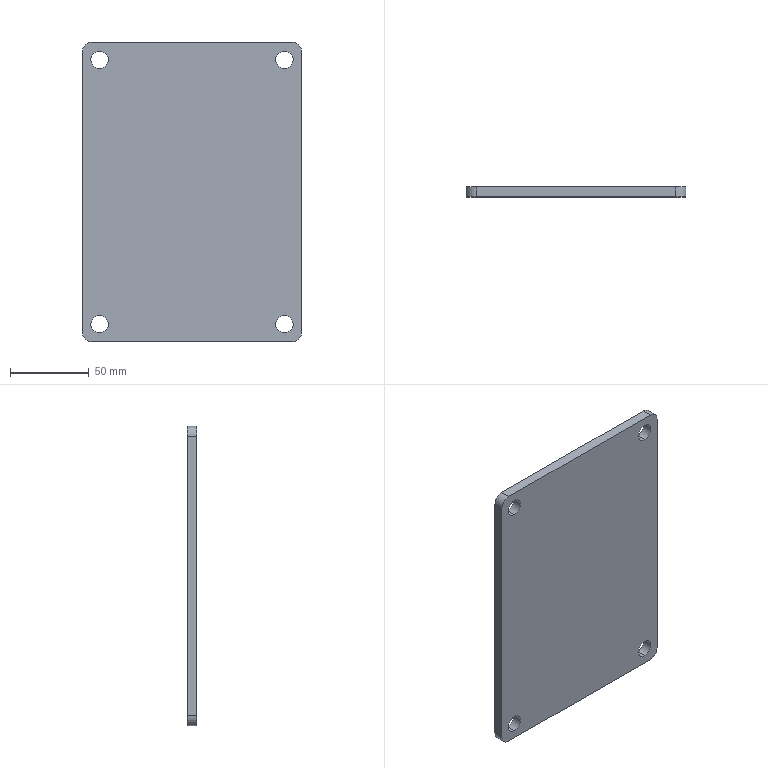Part | SolidWorks | features Extrusion 1, Fillet 1, HoleWzd 1, LPattern 1 | 1 solid | 18 faces | box 139.7 x 6.35 x 190.5 mm | volume 166308 mm3 | cylinder 12 | plane 6 | commonest cylinder face diameters 11.112 x8 12.7 x4
STEP:
#1=CARTESIAN_POINT('',(58.737,0.,78.581));
#2=VERTEX_POINT('',#1);
#3=CARTESIAN_POINT('',(58.737,0.,89.693));
#4=VERTEX_POINT('',#3);
#5=CARTESIAN_POINT('',(58.737,0.,84.137));
#6=DIRECTION('',(0.,1.,0.));
#7=DIRECTION('',(0.,0.,1.));
#8=AXIS2_PLACEMENT_3D('',#5,#6,#7);
#9=CIRCLE('',#8,5.556);
#10=EDGE_CURVE('',#2,#4,#9,.T.);
#11=ORIENTED_EDGE('',*,*,#10,.F.);
#12=CARTESIAN_POINT('',(58.737,6.35,78.581));
#13=VERTEX_POINT('',#12);
#14=CARTESIAN_POINT('',(58.737,6.35,78.581));
#15=DIRECTION('',(0.,1.,0.));
#16=VECTOR('',#15,1000.);
#17=LINE('',#14,#16);
#18=EDGE_CURVE('',#2,#13,#17,.T.);
#19=ORIENTED_EDGE('',*,*,#18,.T.);
#20=CARTESIAN_POINT('',(58.737,6.35,89.693));
#21=VERTEX_POINT('',#20);
#22=CARTESIAN_POINT('',(58.737,6.35,84.137));
#23=DIRECTION('',(0.,1.,0.));
#24=DIRECTION('',(0.,0.,1.));
#25=AXIS2_PLACEMENT_3D('',#22,#23,#24);
#26=CIRCLE('',#25,5.556);
#27=EDGE_CURVE('',#13,#21,#26,.T.);
#28=ORIENTED_EDGE('',*,*,#27,.T.);
#29=CARTESIAN_POINT('',(58.737,6.35,89.693));
#30=DIRECTION('',(0.,1.,0.));
#31=VECTOR('',#30,1000.);
#32=LINE('',#29,#31);
#33=EDGE_CURVE('',#4,#21,#32,.T.);
#34=ORIENTED_EDGE('',*,*,#33,.F.);
#35=EDGE_LOOP('',(#11,#19,#28,#34));
#36=FACE_OUTER_BOUND('',#35,.T.);
#37=CARTESIAN_POINT('',(58.737,6.35,84.137));
#38=DIRECTION('',(0.,1.,0.));
#39=DIRECTION('',(0.,0.,1.));
#40=AXIS2_PLACEMENT_3D('',#37,#38,#39);
#41=CYLINDRICAL_SURFACE('',#40,5.556);
#42=ADVANCED_FACE('',(#36),#41,.F.);
#43=CARTESIAN_POINT('',(-58.738,0.,78.581));
#44=VERTEX_POINT('',#43);
#45=CARTESIAN_POINT('',(-58.738,0.,89.693));
#46=VERTEX_POINT('',#45);
#47=CARTESIAN_POINT('',(-58.738,0.,84.137));
#48=DIRECTION('',(0.,1.,0.));
#49=DIRECTION('',(0.,0.,1.));
#50=AXIS2_PLACEMENT_3D('',#47,#48,#49);
#51=CIRCLE('',#50,5.556);
#52=EDGE_CURVE('',#44,#46,#51,.T.);
#53=ORIENTED_EDGE('',*,*,#52,.F.);
#54=CARTESIAN_POINT('',(-58.738,6.35,78.581));
#55=VERTEX_POINT('',#54);
#56=CARTESIAN_POINT('',(-58.738,6.35,78.581));
#57=DIRECTION('',(0.,1.,0.));
#58=VECTOR('',#57,1000.);
#59=LINE('',#56,#58);
#60=EDGE_CURVE('',#44,#55,#59,.T.);
#61=ORIENTED_EDGE('',*,*,#60,.T.);
#62=CARTESIAN_POINT('',(-58.738,6.35,89.693));
#63=VERTEX_POINT('',#62);
#64=CARTESIAN_POINT('',(-58.738,6.35,84.137));
#65=DIRECTION('',(0.,1.,0.));
#66=DIRECTION('',(0.,0.,1.));
#67=AXIS2_PLACEMENT_3D('',#64,#65,#66);
#68=CIRCLE('',#67,5.556);
#69=EDGE_CURVE('',#55,#63,#68,.T.);
#70=ORIENTED_EDGE('',*,*,#69,.T.);
#71=CARTESIAN_POINT('',(-58.738,6.35,89.693));
#72=DIRECTION('',(0.,1.,0.));
#73=VECTOR('',#72,1000.);
#74=LINE('',#71,#73);
#75=EDGE_CURVE('',#46,#63,#74,.T.);
#76=ORIENTED_EDGE('',*,*,#75,.F.);
#77=EDGE_LOOP('',(#53,#61,#70,#76));
#78=FACE_OUTER_BOUND('',#77,.T.);
#79=CARTESIAN_POINT('',(-58.738,6.35,84.137));
#80=DIRECTION('',(0.,1.,0.));
#81=DIRECTION('',(0.,0.,1.));
#82=AXIS2_PLACEMENT_3D('',#79,#80,#81);
#83=CYLINDRICAL_SURFACE('',#82,5.556);
#84=ADVANCED_FACE('',(#78),#83,.F.);
#85=CARTESIAN_POINT('',(58.737,0.,-89.694));
#86=VERTEX_POINT('',#85);
#87=CARTESIAN_POINT('',(58.737,0.,-78.582));
#88=VERTEX_POINT('',#87);
#89=CARTESIAN_POINT('',(58.737,0.,-84.138));
#90=DIRECTION('',(0.,1.,0.));
#91=DIRECTION('',(0.,0.,1.));
#92=AXIS2_PLACEMENT_3D('',#89,#90,#91);
#93=CIRCLE('',#92,5.556);
#94=EDGE_CURVE('',#86,#88,#93,.T.);
#95=ORIENTED_EDGE('',*,*,#94,.F.);
#96=CARTESIAN_POINT('',(58.737,6.35,-89.694));
#97=VERTEX_POINT('',#96);
#98=CARTESIAN_POINT('',(58.737,6.35,-89.694));
#99=DIRECTION('',(0.,1.,0.));
#100=VECTOR('',#99,1000.);
#101=LINE('',#98,#100);
#102=EDGE_CURVE('',#86,#97,#101,.T.);
#103=ORIENTED_EDGE('',*,*,#102,.T.);
#104=CARTESIAN_POINT('',(58.737,6.35,-78.582));
#105=VERTEX_POINT('',#104);
#106=CARTESIAN_POINT('',(58.737,6.35,-84.138));
#107=DIRECTION('',(0.,1.,0.));
#108=DIRECTION('',(0.,0.,1.));
#109=AXIS2_PLACEMENT_3D('',#106,#107,#108);
#110=CIRCLE('',#109,5.556);
#111=EDGE_CURVE('',#97,#105,#110,.T.);
#112=ORIENTED_EDGE('',*,*,#111,.T.);
#113=CARTESIAN_POINT('',(58.737,6.35,-78.582));
#114=DIRECTION('',(0.,1.,0.));
#115=VECTOR('',#114,1000.);
#116=LINE('',#113,#115);
#117=EDGE_CURVE('',#88,#105,#116,.T.);
#118=ORIENTED_EDGE('',*,*,#117,.F.);
#119=EDGE_LOOP('',(#95,#103,#112,#118));
#120=FACE_OUTER_BOUND('',#119,.T.);
#121=CARTESIAN_POINT('',(58.737,6.35,-84.138));
#122=DIRECTION('',(0.,1.,0.));
#123=DIRECTION('',(0.,0.,1.));
#124=AXIS2_PLACEMENT_3D('',#121,#122,#123);
#125=CYLINDRICAL_SURFACE('',#124,5.556);
#126=ADVANCED_FACE('',(#120),#125,.F.);
#127=CARTESIAN_POINT('',(-58.738,0.,-89.694));
#128=VERTEX_POINT('',#127);
#129=CARTESIAN_POINT('',(-58.738,0.,-78.582));
#130=VERTEX_POINT('',#129);
#131=CARTESIAN_POINT('',(-58.738,0.,-84.138));
#132=DIRECTION('',(0.,1.,0.));
#133=DIRECTION('',(0.,0.,1.));
#134=AXIS2_PLACEMENT_3D('',#131,#132,#133);
#135=CIRCLE('',#134,5.556);
#136=EDGE_CURVE('',#128,#130,#135,.T.);
#137=ORIENTED_EDGE('',*,*,#136,.F.);
#138=CARTESIAN_POINT('',(-58.738,6.35,-89.694));
#139=VERTEX_POINT('',#138);
#140=CARTESIAN_POINT('',(-58.738,6.35,-89.694));
#141=DIRECTION('',(0.,1.,0.));
#142=VECTOR('',#141,1000.);
#143=LINE('',#140,#142);
#144=EDGE_CURVE('',#128,#139,#143,.T.);
#145=ORIENTED_EDGE('',*,*,#144,.T.);
#146=CARTESIAN_POINT('',(-58.738,6.35,-78.582));
#147=VERTEX_POINT('',#146);
#148=CARTESIAN_POINT('',(-58.738,6.35,-84.138));
#149=DIRECTION('',(0.,1.,0.));
#150=DIRECTION('',(0.,0.,1.));
#151=AXIS2_PLACEMENT_3D('',#148,#149,#150);
#152=CIRCLE('',#151,5.556);
#153=EDGE_CURVE('',#139,#147,#152,.T.);
#154=ORIENTED_EDGE('',*,*,#153,.T.);
#155=CARTESIAN_POINT('',(-58.738,6.35,-78.582));
#156=DIRECTION('',(0.,1.,0.));
#157=VECTOR('',#156,1000.);
#158=LINE('',#155,#157);
#159=EDGE_CURVE('',#130,#147,#158,.T.);
#160=ORIENTED_EDGE('',*,*,#159,.F.);
#161=EDGE_LOOP('',(#137,#145,#154,#160));
#162=FACE_OUTER_BOUND('',#161,.T.);
#163=CARTESIAN_POINT('',(-58.738,6.35,-84.138));
#164=DIRECTION('',(0.,1.,0.));
#165=DIRECTION('',(0.,0.,1.));
#166=AXIS2_PLACEMENT_3D('',#163,#164,#165);
#167=CYLINDRICAL_SURFACE('',#166,5.556);
#168=ADVANCED_FACE('',(#162),#167,.F.);
#169=CARTESIAN_POINT('',(-69.85,6.35,-88.9));
#170=VERTEX_POINT('',#169);
#171=CARTESIAN_POINT('',(-69.85,6.35,88.9));
#172=VERTEX_POINT('',#171);
#173=CARTESIAN_POINT('',(-69.85,6.35,-95.25));
#174=DIRECTION('',(0.,0.,1.));
#175=VECTOR('',#174,1000.);
#176=LINE('',#173,#175);
#177=EDGE_CURVE('',#170,#172,#176,.T.);
#178=ORIENTED_EDGE('',*,*,#177,.F.);
#179=CARTESIAN_POINT('',(-69.85,0.,-88.9));
#180=VERTEX_POINT('',#179);
#181=CARTESIAN_POINT('',(-69.85,6.35,-88.9));
#182=DIRECTION('',(0.,-1.,0.));
#183=VECTOR('',#182,1000.);
#184=LINE('',#181,#183);
#185=EDGE_CURVE('',#170,#180,#184,.T.);
#186=ORIENTED_EDGE('',*,*,#185,.T.);
#187=CARTESIAN_POINT('',(-69.85,0.,88.9));
#188=VERTEX_POINT('',#187);
#189=CARTESIAN_POINT('',(-69.85,0.,-95.25));
#190=DIRECTION('',(0.,0.,1.));
#191=VECTOR('',#190,1000.);
#192=LINE('',#189,#191);
#193=EDGE_CURVE('',#180,#188,#192,.T.);
#194=ORIENTED_EDGE('',*,*,#193,.T.);
#195=CARTESIAN_POINT('',(-69.85,6.35,88.9));
#196=DIRECTION('',(0.,1.,0.));
#197=VECTOR('',#196,1000.);
#198=LINE('',#195,#197);
#199=EDGE_CURVE('',#188,#172,#198,.T.);
#200=ORIENTED_EDGE('',*,*,#199,.T.);
#201=EDGE_LOOP('',(#178,#186,#194,#200));
#202=FACE_OUTER_BOUND('',#201,.T.);
#203=CARTESIAN_POINT('',(-69.85,6.35,-95.25));
#204=DIRECTION('',(1.,0.,0.));
#205=DIRECTION('',(0.,0.,-1.));
#206=AXIS2_PLACEMENT_3D('',#203,#204,#205);
#207=PLANE('',#206);
#208=ADVANCED_FACE('',(#202),#207,.F.);
#209=CARTESIAN_POINT('',(-63.5,0.,95.25));
#210=VERTEX_POINT('',#209);
#211=CARTESIAN_POINT('',(63.5,0.,95.25));
#212=VERTEX_POINT('',#211);
#213=CARTESIAN_POINT('',(-69.85,0.,95.25));
#214=DIRECTION('',(1.,0.,0.));
#215=VECTOR('',#214,1000.);
#216=LINE('',#213,#215);
#217=EDGE_CURVE('',#210,#212,#216,.T.);
#218=ORIENTED_EDGE('',*,*,#217,.T.);
#219=CARTESIAN_POINT('',(63.5,6.35,95.25));
#220=VERTEX_POINT('',#219);
#221=CARTESIAN_POINT('',(63.5,6.35,95.25));
#222=DIRECTION('',(0.,1.,0.));
#223=VECTOR('',#222,1000.);
#224=LINE('',#221,#223);
#225=EDGE_CURVE('',#212,#220,#224,.T.);
#226=ORIENTED_EDGE('',*,*,#225,.T.);
#227=CARTESIAN_POINT('',(-63.5,6.35,95.25));
#228=VERTEX_POINT('',#227);
#229=CARTESIAN_POINT('',(-69.85,6.35,95.25));
#230=DIRECTION('',(1.,0.,0.));
#231=VECTOR('',#230,1000.);
#232=LINE('',#229,#231);
#233=EDGE_CURVE('',#228,#220,#232,.T.);
#234=ORIENTED_EDGE('',*,*,#233,.F.);
#235=CARTESIAN_POINT('',(-63.5,6.35,95.25));
#236=DIRECTION('',(0.,-1.,0.));
#237=VECTOR('',#236,1000.);
#238=LINE('',#235,#237);
#239=EDGE_CURVE('',#228,#210,#238,.T.);
#240=ORIENTED_EDGE('',*,*,#239,.T.);
#241=EDGE_LOOP('',(#218,#226,#234,#240));
#242=FACE_OUTER_BOUND('',#241,.T.);
#243=CARTESIAN_POINT('',(-69.85,6.35,95.25));
#244=DIRECTION('',(0.,0.,-1.));
#245=DIRECTION('',(-1.,0.,0.));
#246=AXIS2_PLACEMENT_3D('',#243,#244,#245);
#247=PLANE('',#246);
#248=ADVANCED_FACE('',(#242),#247,.F.);
#249=CARTESIAN_POINT('',(69.85,0.,88.9));
#250=VERTEX_POINT('',#249);
#251=CARTESIAN_POINT('',(69.85,0.,-88.9));
#252=VERTEX_POINT('',#251);
#253=CARTESIAN_POINT('',(69.85,0.,-95.25));
#254=DIRECTION('',(0.,0.,-1.));
#255=VECTOR('',#254,1000.);
#256=LINE('',#253,#255);
#257=EDGE_CURVE('',#250,#252,#256,.T.);
#258=ORIENTED_EDGE('',*,*,#257,.T.);
#259=CARTESIAN_POINT('',(69.85,6.35,-88.9));
#260=VERTEX_POINT('',#259);
#261=CARTESIAN_POINT('',(69.85,6.35,-88.9));
#262=DIRECTION('',(0.,1.,0.));
#263=VECTOR('',#262,1000.);
#264=LINE('',#261,#263);
#265=EDGE_CURVE('',#252,#260,#264,.T.);
#266=ORIENTED_EDGE('',*,*,#265,.T.);
#267=CARTESIAN_POINT('',(69.85,6.35,88.9));
#268=VERTEX_POINT('',#267);
#269=CARTESIAN_POINT('',(69.85,6.35,-95.25));
#270=DIRECTION('',(0.,0.,-1.));
#271=VECTOR('',#270,1000.);
#272=LINE('',#269,#271);
#273=EDGE_CURVE('',#268,#260,#272,.T.);
#274=ORIENTED_EDGE('',*,*,#273,.F.);
#275=CARTESIAN_POINT('',(69.85,6.35,88.9));
#276=DIRECTION('',(0.,-1.,0.));
#277=VECTOR('',#276,1000.);
#278=LINE('',#275,#277);
#279=EDGE_CURVE('',#268,#250,#278,.T.);
#280=ORIENTED_EDGE('',*,*,#279,.T.);
#281=EDGE_LOOP('',(#258,#266,#274,#280));
#282=FACE_OUTER_BOUND('',#281,.T.);
#283=CARTESIAN_POINT('',(69.85,6.35,-95.25));
#284=DIRECTION('',(-1.,0.,0.));
#285=DIRECTION('',(0.,0.,1.));
#286=AXIS2_PLACEMENT_3D('',#283,#284,#285);
#287=PLANE('',#286);
#288=ADVANCED_FACE('',(#282),#287,.F.);
#289=CARTESIAN_POINT('',(63.5,0.,-95.25));
#290=VERTEX_POINT('',#289);
#291=CARTESIAN_POINT('',(-63.5,0.,-95.25));
#292=VERTEX_POINT('',#291);
#293=CARTESIAN_POINT('',(-69.85,0.,-95.25));
#294=DIRECTION('',(-1.,0.,0.));
#295=VECTOR('',#294,1000.);
#296=LINE('',#293,#295);
#297=EDGE_CURVE('',#290,#292,#296,.T.);
#298=ORIENTED_EDGE('',*,*,#297,.T.);
#299=CARTESIAN_POINT('',(-63.5,6.35,-95.25));
#300=VERTEX_POINT('',#299);
#301=CARTESIAN_POINT('',(-63.5,6.35,-95.25));
#302=DIRECTION('',(0.,1.,0.));
#303=VECTOR('',#302,1000.);
#304=LINE('',#301,#303);
#305=EDGE_CURVE('',#292,#300,#304,.T.);
#306=ORIENTED_EDGE('',*,*,#305,.T.);
#307=CARTESIAN_POINT('',(63.5,6.35,-95.25));
#308=VERTEX_POINT('',#307);
#309=CARTESIAN_POINT('',(-69.85,6.35,-95.25));
#310=DIRECTION('',(-1.,0.,0.));
#311=VECTOR('',#310,1000.);
#312=LINE('',#309,#311);
#313=EDGE_CURVE('',#308,#300,#312,.T.);
#314=ORIENTED_EDGE('',*,*,#313,.F.);
#315=CARTESIAN_POINT('',(63.5,6.35,-95.25));
#316=DIRECTION('',(0.,-1.,0.));
#317=VECTOR('',#316,1000.);
#318=LINE('',#315,#317);
#319=EDGE_CURVE('',#308,#290,#318,.T.);
#320=ORIENTED_EDGE('',*,*,#319,.T.);
#321=EDGE_LOOP('',(#298,#306,#314,#320));
#322=FACE_OUTER_BOUND('',#321,.T.);
#323=CARTESIAN_POINT('',(-69.85,6.35,-95.25));
#324=DIRECTION('',(0.,0.,1.));
#325=DIRECTION('',(1.,0.,0.));
#326=AXIS2_PLACEMENT_3D('',#323,#324,#325);
#327=PLANE('',#326);
#328=ADVANCED_FACE('',(#322),#327,.F.);
#329=CARTESIAN_POINT('',(58.737,6.35,84.137));
#330=DIRECTION('',(0.,1.,0.));
#331=DIRECTION('',(0.,0.,1.));
#332=AXIS2_PLACEMENT_3D('',#329,#330,#331);
#333=CIRCLE('',#332,5.556);
#334=EDGE_CURVE('',#21,#13,#333,.T.);
#335=ORIENTED_EDGE('',*,*,#334,.F.);
#336=ORIENTED_EDGE('',*,*,#27,.F.);
#337=EDGE_LOOP('',(#335,#336));
#338=FACE_BOUND('',#337,.T.);
#339=CARTESIAN_POINT('',(-58.738,6.35,84.137));
#340=DIRECTION('',(0.,1.,0.));
#341=DIRECTION('',(0.,0.,1.));
#342=AXIS2_PLACEMENT_3D('',#339,#340,#341);
#343=CIRCLE('',#342,5.556);
#344=EDGE_CURVE('',#63,#55,#343,.T.);
#345=ORIENTED_EDGE('',*,*,#344,.F.);
#346=ORIENTED_EDGE('',*,*,#69,.F.);
#347=EDGE_LOOP('',(#345,#346));
#348=FACE_BOUND('',#347,.T.);
#349=CARTESIAN_POINT('',(58.737,6.35,-84.138));
#350=DIRECTION('',(0.,1.,0.));
#351=DIRECTION('',(0.,0.,1.));
#352=AXIS2_PLACEMENT_3D('',#349,#350,#351);
#353=CIRCLE('',#352,5.556);
#354=EDGE_CURVE('',#105,#97,#353,.T.);
#355=ORIENTED_EDGE('',*,*,#354,.F.);
#356=ORIENTED_EDGE('',*,*,#111,.F.);
#357=EDGE_LOOP('',(#355,#356));
#358=FACE_BOUND('',#357,.T.);
#359=CARTESIAN_POINT('',(-58.738,6.35,-84.138));
#360=DIRECTION('',(0.,1.,0.));
#361=DIRECTION('',(0.,0.,1.));
#362=AXIS2_PLACEMENT_3D('',#359,#360,#361);
#363=CIRCLE('',#362,5.556);
#364=EDGE_CURVE('',#147,#139,#363,.T.);
#365=ORIENTED_EDGE('',*,*,#364,.F.);
#366=ORIENTED_EDGE('',*,*,#153,.F.);
#367=EDGE_LOOP('',(#365,#366));
#368=FACE_BOUND('',#367,.T.);
#369=ORIENTED_EDGE('',*,*,#313,.T.);
#370=CARTESIAN_POINT('',(-63.5,6.35,-88.9));
#371=DIRECTION('',(0.,1.,0.));
#372=DIRECTION('',(0.,0.,1.));
#373=AXIS2_PLACEMENT_3D('',#370,#371,#372);
#374=CIRCLE('',#373,6.35);
#375=EDGE_CURVE('',#300,#170,#374,.T.);
#376=ORIENTED_EDGE('',*,*,#375,.T.);
#377=ORIENTED_EDGE('',*,*,#177,.T.);
#378=CARTESIAN_POINT('',(-63.5,6.35,88.9));
#379=DIRECTION('',(0.,1.,0.));
#380=DIRECTION('',(0.,0.,1.));
#381=AXIS2_PLACEMENT_3D('',#378,#379,#380);
#382=CIRCLE('',#381,6.35);
#383=EDGE_CURVE('',#172,#228,#382,.T.);
#384=ORIENTED_EDGE('',*,*,#383,.T.);
#385=ORIENTED_EDGE('',*,*,#233,.T.);
#386=CARTESIAN_POINT('',(63.5,6.35,88.9));
#387=DIRECTION('',(0.,1.,0.));
#388=DIRECTION('',(0.,0.,1.));
#389=AXIS2_PLACEMENT_3D('',#386,#387,#388);
#390=CIRCLE('',#389,6.35);
#391=EDGE_CURVE('',#220,#268,#390,.T.);
#392=ORIENTED_EDGE('',*,*,#391,.T.);
#393=ORIENTED_EDGE('',*,*,#273,.T.);
#394=CARTESIAN_POINT('',(63.5,6.35,-88.9));
#395=DIRECTION('',(0.,1.,0.));
#396=DIRECTION('',(0.,0.,1.));
#397=AXIS2_PLACEMENT_3D('',#394,#395,#396);
#398=CIRCLE('',#397,6.35);
#399=EDGE_CURVE('',#260,#308,#398,.T.);
#400=ORIENTED_EDGE('',*,*,#399,.T.);
#401=EDGE_LOOP('',(#369,#376,#377,#384,#385,#392,#393,#400));
#402=FACE_OUTER_BOUND('',#401,.T.);
#403=CARTESIAN_POINT('',(0.,6.35,0.));
#404=DIRECTION('',(0.,1.,0.));
#405=DIRECTION('',(0.,0.,1.));
#406=AXIS2_PLACEMENT_3D('',#403,#404,#405);
#407=PLANE('',#406);
#408=ADVANCED_FACE('',(#338,#348,#358,#368,#402),#407,.T.);
#409=CARTESIAN_POINT('',(58.737,0.,84.137));
#410=DIRECTION('',(0.,1.,0.));
#411=DIRECTION('',(0.,0.,1.));
#412=AXIS2_PLACEMENT_3D('',#409,#410,#411);
#413=CIRCLE('',#412,5.556);
#414=EDGE_CURVE('',#4,#2,#413,.T.);
#415=ORIENTED_EDGE('',*,*,#414,.T.);
#416=ORIENTED_EDGE('',*,*,#10,.T.);
#417=EDGE_LOOP('',(#415,#416));
#418=FACE_BOUND('',#417,.T.);
#419=CARTESIAN_POINT('',(-58.738,0.,84.137));
#420=DIRECTION('',(0.,1.,0.));
#421=DIRECTION('',(0.,0.,1.));
#422=AXIS2_PLACEMENT_3D('',#419,#420,#421);
#423=CIRCLE('',#422,5.556);
#424=EDGE_CURVE('',#46,#44,#423,.T.);
#425=ORIENTED_EDGE('',*,*,#424,.T.);
#426=ORIENTED_EDGE('',*,*,#52,.T.);
#427=EDGE_LOOP('',(#425,#426));
#428=FACE_BOUND('',#427,.T.);
#429=CARTESIAN_POINT('',(58.737,0.,-84.138));
#430=DIRECTION('',(0.,1.,0.));
#431=DIRECTION('',(0.,0.,1.));
#432=AXIS2_PLACEMENT_3D('',#429,#430,#431);
#433=CIRCLE('',#432,5.556);
#434=EDGE_CURVE('',#88,#86,#433,.T.);
#435=ORIENTED_EDGE('',*,*,#434,.T.);
#436=ORIENTED_EDGE('',*,*,#94,.T.);
#437=EDGE_LOOP('',(#435,#436));
#438=FACE_BOUND('',#437,.T.);
#439=CARTESIAN_POINT('',(-58.738,0.,-84.138));
#440=DIRECTION('',(0.,1.,0.));
#441=DIRECTION('',(0.,0.,1.));
#442=AXIS2_PLACEMENT_3D('',#439,#440,#441);
#443=CIRCLE('',#442,5.556);
#444=EDGE_CURVE('',#130,#128,#443,.T.);
#445=ORIENTED_EDGE('',*,*,#444,.T.);
#446=ORIENTED_EDGE('',*,*,#136,.T.);
#447=EDGE_LOOP('',(#445,#446));
#448=FACE_BOUND('',#447,.T.);
#449=ORIENTED_EDGE('',*,*,#193,.F.);
#450=CARTESIAN_POINT('',(-63.5,0.,-88.9));
#451=DIRECTION('',(0.,-1.,0.));
#452=DIRECTION('',(0.,0.,1.));
#453=AXIS2_PLACEMENT_3D('',#450,#451,#452);
#454=CIRCLE('',#453,6.35);
#455=EDGE_CURVE('',#180,#292,#454,.T.);
#456=ORIENTED_EDGE('',*,*,#455,.T.);
#457=ORIENTED_EDGE('',*,*,#297,.F.);
#458=CARTESIAN_POINT('',(63.5,0.,-88.9));
#459=DIRECTION('',(0.,-1.,0.));
#460=DIRECTION('',(0.,0.,1.));
#461=AXIS2_PLACEMENT_3D('',#458,#459,#460);
#462=CIRCLE('',#461,6.35);
#463=EDGE_CURVE('',#290,#252,#462,.T.);
#464=ORIENTED_EDGE('',*,*,#463,.T.);
#465=ORIENTED_EDGE('',*,*,#257,.F.);
#466=CARTESIAN_POINT('',(63.5,0.,88.9));
#467=DIRECTION('',(0.,-1.,0.));
#468=DIRECTION('',(0.,0.,1.));
#469=AXIS2_PLACEMENT_3D('',#466,#467,#468);
#470=CIRCLE('',#469,6.35);
#471=EDGE_CURVE('',#250,#212,#470,.T.);
#472=ORIENTED_EDGE('',*,*,#471,.T.);
#473=ORIENTED_EDGE('',*,*,#217,.F.);
#474=CARTESIAN_POINT('',(-63.5,0.,88.9));
#475=DIRECTION('',(0.,-1.,0.));
#476=DIRECTION('',(0.,0.,1.));
#477=AXIS2_PLACEMENT_3D('',#474,#475,#476);
#478=CIRCLE('',#477,6.35);
#479=EDGE_CURVE('',#210,#188,#478,.T.);
#480=ORIENTED_EDGE('',*,*,#479,.T.);
#481=EDGE_LOOP('',(#449,#456,#457,#464,#465,#472,#473,#480));
#482=FACE_OUTER_BOUND('',#481,.T.);
#483=CARTESIAN_POINT('',(0.,0.,0.));
#484=DIRECTION('',(0.,1.,0.));
#485=DIRECTION('',(0.,0.,1.));
#486=AXIS2_PLACEMENT_3D('',#483,#484,#485);
#487=PLANE('',#486);
#488=ADVANCED_FACE('',(#418,#428,#438,#448,#482),#487,.F.);
#489=ORIENTED_EDGE('',*,*,#375,.F.);
#490=ORIENTED_EDGE('',*,*,#305,.F.);
#491=ORIENTED_EDGE('',*,*,#455,.F.);
#492=ORIENTED_EDGE('',*,*,#185,.F.);
#493=EDGE_LOOP('',(#489,#490,#491,#492));
#494=FACE_OUTER_BOUND('',#493,.T.);
#495=CARTESIAN_POINT('',(-63.5,6.35,-88.9));
#496=DIRECTION('',(0.,-1.,0.));
#497=DIRECTION('',(0.,0.,-1.));
#498=AXIS2_PLACEMENT_3D('',#495,#496,#497);
#499=CYLINDRICAL_SURFACE('',#498,6.35);
#500=ADVANCED_FACE('',(#494),#499,.T.);
#501=ORIENTED_EDGE('',*,*,#399,.F.);
#502=ORIENTED_EDGE('',*,*,#265,.F.);
#503=ORIENTED_EDGE('',*,*,#463,.F.);
#504=ORIENTED_EDGE('',*,*,#319,.F.);
#505=EDGE_LOOP('',(#501,#502,#503,#504));
#506=FACE_OUTER_BOUND('',#505,.T.);
#507=CARTESIAN_POINT('',(63.5,6.35,-88.9));
#508=DIRECTION('',(0.,-1.,0.));
#509=DIRECTION('',(0.,0.,-1.));
#510=AXIS2_PLACEMENT_3D('',#507,#508,#509);
#511=CYLINDRICAL_SURFACE('',#510,6.35);
#512=ADVANCED_FACE('',(#506),#511,.T.);
#513=ORIENTED_EDGE('',*,*,#391,.F.);
#514=ORIENTED_EDGE('',*,*,#225,.F.);
#515=ORIENTED_EDGE('',*,*,#471,.F.);
#516=ORIENTED_EDGE('',*,*,#279,.F.);
#517=EDGE_LOOP('',(#513,#514,#515,#516));
#518=FACE_OUTER_BOUND('',#517,.T.);
#519=CARTESIAN_POINT('',(63.5,6.35,88.9));
#520=DIRECTION('',(0.,-1.,0.));
#521=DIRECTION('',(0.,0.,-1.));
#522=AXIS2_PLACEMENT_3D('',#519,#520,#521);
#523=CYLINDRICAL_SURFACE('',#522,6.35);
#524=ADVANCED_FACE('',(#518),#523,.T.);
#525=ORIENTED_EDGE('',*,*,#383,.F.);
#526=ORIENTED_EDGE('',*,*,#199,.F.);
#527=ORIENTED_EDGE('',*,*,#479,.F.);
#528=ORIENTED_EDGE('',*,*,#239,.F.);
#529=EDGE_LOOP('',(#525,#526,#527,#528));
#530=FACE_OUTER_BOUND('',#529,.T.);
#531=CARTESIAN_POINT('',(-63.5,6.35,88.9));
#532=DIRECTION('',(0.,-1.,0.));
#533=DIRECTION('',(0.,0.,-1.));
#534=AXIS2_PLACEMENT_3D('',#531,#532,#533);
#535=CYLINDRICAL_SURFACE('',#534,6.35);
#536=ADVANCED_FACE('',(#530),#535,.T.);
#537=ORIENTED_EDGE('',*,*,#144,.F.);
#538=ORIENTED_EDGE('',*,*,#444,.F.);
#539=ORIENTED_EDGE('',*,*,#159,.T.);
#540=ORIENTED_EDGE('',*,*,#364,.T.);
#541=EDGE_LOOP('',(#537,#538,#539,#540));
#542=FACE_OUTER_BOUND('',#541,.T.);
#543=CARTESIAN_POINT('',(-58.738,6.35,-84.138));
#544=DIRECTION('',(0.,1.,0.));
#545=DIRECTION('',(0.,0.,1.));
#546=AXIS2_PLACEMENT_3D('',#543,#544,#545);
#547=CYLINDRICAL_SURFACE('',#546,5.556);
#548=ADVANCED_FACE('',(#542),#547,.F.);
#549=ORIENTED_EDGE('',*,*,#102,.F.);
#550=ORIENTED_EDGE('',*,*,#434,.F.);
#551=ORIENTED_EDGE('',*,*,#117,.T.);
#552=ORIENTED_EDGE('',*,*,#354,.T.);
#553=EDGE_LOOP('',(#549,#550,#551,#552));
#554=FACE_OUTER_BOUND('',#553,.T.);
#555=CARTESIAN_POINT('',(58.737,6.35,-84.138));
#556=DIRECTION('',(0.,1.,0.));
#557=DIRECTION('',(0.,0.,1.));
#558=AXIS2_PLACEMENT_3D('',#555,#556,#557);
#559=CYLINDRICAL_SURFACE('',#558,5.556);
#560=ADVANCED_FACE('',(#554),#559,.F.);
#561=ORIENTED_EDGE('',*,*,#60,.F.);
#562=ORIENTED_EDGE('',*,*,#424,.F.);
#563=ORIENTED_EDGE('',*,*,#75,.T.);
#564=ORIENTED_EDGE('',*,*,#344,.T.);
#565=EDGE_LOOP('',(#561,#562,#563,#564));
#566=FACE_OUTER_BOUND('',#565,.T.);
#567=CARTESIAN_POINT('',(-58.738,6.35,84.137));
#568=DIRECTION('',(0.,1.,0.));
#569=DIRECTION('',(0.,0.,1.));
#570=AXIS2_PLACEMENT_3D('',#567,#568,#569);
#571=CYLINDRICAL_SURFACE('',#570,5.556);
#572=ADVANCED_FACE('',(#566),#571,.F.);
#573=ORIENTED_EDGE('',*,*,#18,.F.);
#574=ORIENTED_EDGE('',*,*,#414,.F.);
#575=ORIENTED_EDGE('',*,*,#33,.T.);
#576=ORIENTED_EDGE('',*,*,#334,.T.);
#577=EDGE_LOOP('',(#573,#574,#575,#576));
#578=FACE_OUTER_BOUND('',#577,.T.);
#579=CARTESIAN_POINT('',(58.737,6.35,84.137));
#580=DIRECTION('',(0.,1.,0.));
#581=DIRECTION('',(0.,0.,1.));
#582=AXIS2_PLACEMENT_3D('',#579,#580,#581);
#583=CYLINDRICAL_SURFACE('',#582,5.556);
#584=ADVANCED_FACE('',(#578),#583,.F.);
#585=CLOSED_SHELL('',(#42,#84,#126,#168,#208,#248,#288,#328,#408,#488,#500,#512,#524,#536,#548,#560,#572,#584));
#586=MANIFOLD_SOLID_BREP('',#585);
#587=CARTESIAN_POINT('',(0.,0.,0.));
#588=DIRECTION('',(0.,0.,1.));
#589=DIRECTION('',(1.,0.,0.));
#590=AXIS2_PLACEMENT_3D('',#587,#588,#589);
#591=(LENGTH_UNIT()NAMED_UNIT(*)SI_UNIT(.MILLI.,.METRE.));
#592=UNCERTAINTY_MEASURE_WITH_UNIT(LENGTH_MEASURE(0.00001),#591,'','');
#593=(NAMED_UNIT(*)PLANE_ANGLE_UNIT()SI_UNIT($,.RADIAN.));
#594=(NAMED_UNIT(*)SI_UNIT($,.STERADIAN.)SOLID_ANGLE_UNIT());
#595=(GEOMETRIC_REPRESENTATION_CONTEXT(3)GLOBAL_UNCERTAINTY_ASSIGNED_CONTEXT((#592))GLOBAL_UNIT_ASSIGNED_CONTEXT((#591,#593,#594))REPRESENTATION_CONTEXT('',''));
#596=ADVANCED_BREP_SHAPE_REPRESENTATION('',(#586,#590),#595);